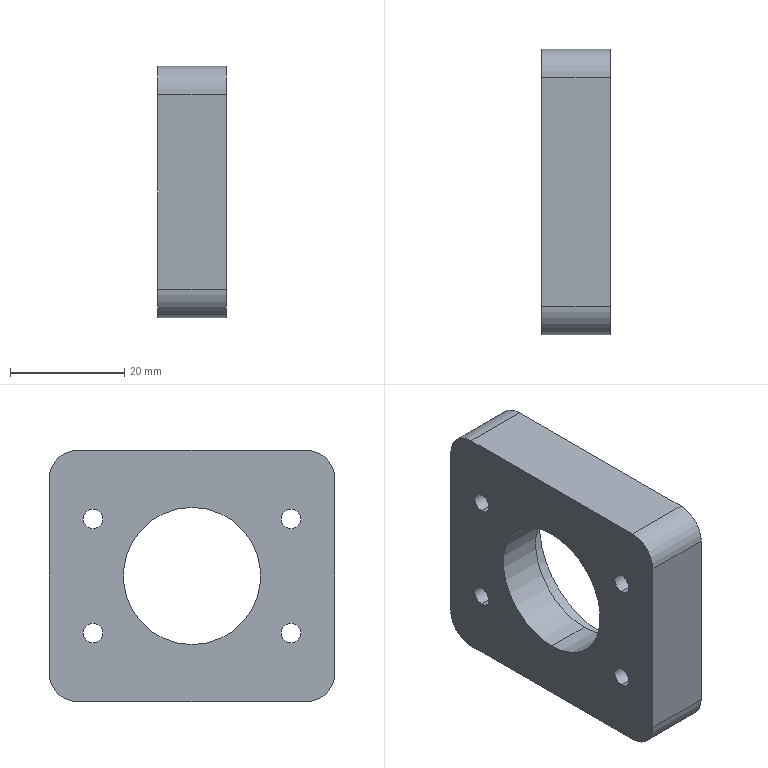Part | STEP file | ASND-0110-TCTF01-28 | 1 solid | 51 faces | box 12 x 50 x 44 mm | volume 18847 mm3 | cylinder 32 | plane 11 | cone 8 | commonest cylinder face diameters 2.5 x8 3.4 x8 6 x8 10 x4 24 x2 30 x2